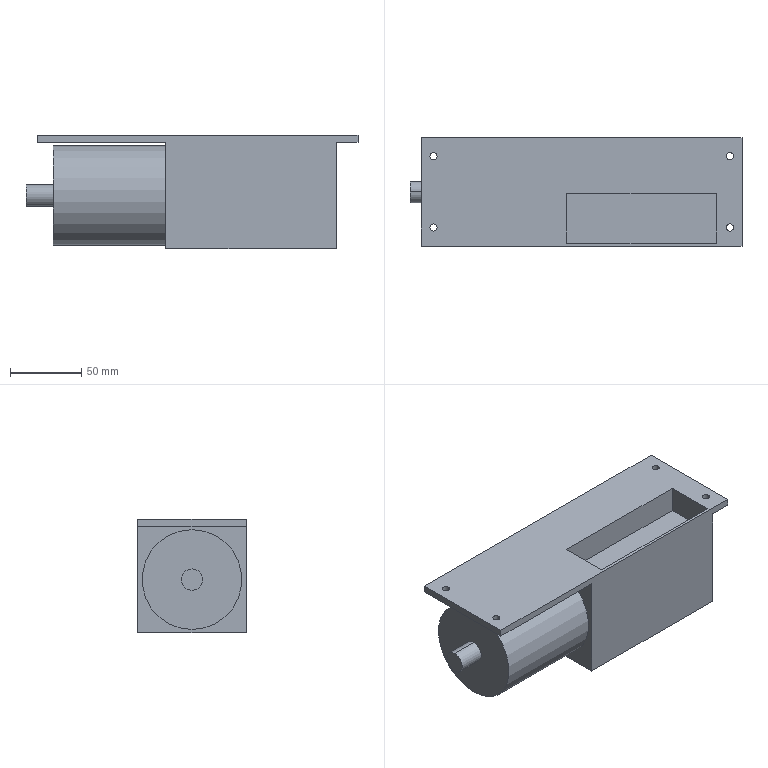Part | 1 solid | 29 faces | box 233 x 76 x 80 mm | volume 1006668 mm3 | plane 17 | cylinder 12 | commonest cylinder face diameters 5 x8 15 x2 70 x2
STEP:
#1=CARTESIAN_POINT('',(-120.5,0.,45.));
#2=VERTEX_POINT('',#1);
#3=CARTESIAN_POINT('',(-120.5,0.,30.));
#4=VERTEX_POINT('',#3);
#5=CARTESIAN_POINT('',(-120.5,0.,37.5));
#6=DIRECTION('',(-1.,0.,0.));
#7=DIRECTION('',(0.,0.,1.));
#8=AXIS2_PLACEMENT_3D('',#5,#6,#7);
#9=CIRCLE('',#8,7.5);
#10=EDGE_CURVE('',#2,#4,#9,.T.);
#11=ORIENTED_EDGE('',*,*,#10,.F.);
#12=CARTESIAN_POINT('',(-101.5,0.,45.));
#13=VERTEX_POINT('',#12);
#14=CARTESIAN_POINT('',(-120.5,0.,45.));
#15=DIRECTION('',(1.,0.,0.));
#16=VECTOR('',#15,1000.);
#17=LINE('',#14,#16);
#18=EDGE_CURVE('',#2,#13,#17,.T.);
#19=ORIENTED_EDGE('',*,*,#18,.T.);
#20=CARTESIAN_POINT('',(-101.5,0.,30.));
#21=VERTEX_POINT('',#20);
#22=CARTESIAN_POINT('',(-101.5,0.,37.5));
#23=DIRECTION('',(-1.,0.,0.));
#24=DIRECTION('',(0.,0.,1.));
#25=AXIS2_PLACEMENT_3D('',#22,#23,#24);
#26=CIRCLE('',#25,7.5);
#27=EDGE_CURVE('',#13,#21,#26,.T.);
#28=ORIENTED_EDGE('',*,*,#27,.T.);
#29=CARTESIAN_POINT('',(-120.5,0.,30.));
#30=DIRECTION('',(1.,0.,0.));
#31=VECTOR('',#30,1000.);
#32=LINE('',#29,#31);
#33=EDGE_CURVE('',#4,#21,#32,.T.);
#34=ORIENTED_EDGE('',*,*,#33,.F.);
#35=EDGE_LOOP('',(#11,#19,#28,#34));
#36=FACE_OUTER_BOUND('',#35,.T.);
#37=CARTESIAN_POINT('',(-120.5,0.,37.5));
#38=DIRECTION('',(1.,0.,0.));
#39=DIRECTION('',(0.,0.,-1.));
#40=AXIS2_PLACEMENT_3D('',#37,#38,#39);
#41=CYLINDRICAL_SURFACE('',#40,7.5);
#42=ADVANCED_FACE('',(#36),#41,.T.);
#43=CARTESIAN_POINT('',(-101.5,0.,72.5));
#44=VERTEX_POINT('',#43);
#45=CARTESIAN_POINT('',(-101.5,0.,2.5));
#46=VERTEX_POINT('',#45);
#47=CARTESIAN_POINT('',(-101.5,0.,37.5));
#48=DIRECTION('',(-1.,0.,0.));
#49=DIRECTION('',(0.,0.,1.));
#50=AXIS2_PLACEMENT_3D('',#47,#48,#49);
#51=CIRCLE('',#50,35.);
#52=EDGE_CURVE('',#44,#46,#51,.T.);
#53=ORIENTED_EDGE('',*,*,#52,.F.);
#54=CARTESIAN_POINT('',(-22.5,0.,72.5));
#55=VERTEX_POINT('',#54);
#56=CARTESIAN_POINT('',(-101.5,0.,72.5));
#57=DIRECTION('',(1.,0.,0.));
#58=VECTOR('',#57,1000.);
#59=LINE('',#56,#58);
#60=EDGE_CURVE('',#44,#55,#59,.T.);
#61=ORIENTED_EDGE('',*,*,#60,.T.);
#62=CARTESIAN_POINT('',(-22.5,0.,2.5));
#63=VERTEX_POINT('',#62);
#64=CARTESIAN_POINT('',(-22.5,0.,37.5));
#65=DIRECTION('',(-1.,0.,0.));
#66=DIRECTION('',(0.,0.,-1.));
#67=AXIS2_PLACEMENT_3D('',#64,#65,#66);
#68=CIRCLE('',#67,35.);
#69=EDGE_CURVE('',#55,#63,#68,.T.);
#70=ORIENTED_EDGE('',*,*,#69,.T.);
#71=CARTESIAN_POINT('',(-101.5,0.,2.5));
#72=DIRECTION('',(1.,0.,0.));
#73=VECTOR('',#72,1000.);
#74=LINE('',#71,#73);
#75=EDGE_CURVE('',#46,#63,#74,.T.);
#76=ORIENTED_EDGE('',*,*,#75,.F.);
#77=EDGE_LOOP('',(#53,#61,#70,#76));
#78=FACE_OUTER_BOUND('',#77,.T.);
#79=CARTESIAN_POINT('',(-101.5,0.,37.5));
#80=DIRECTION('',(1.,0.,0.));
#81=DIRECTION('',(0.,0.,-1.));
#82=AXIS2_PLACEMENT_3D('',#79,#80,#81);
#83=CYLINDRICAL_SURFACE('',#82,35.);
#84=ADVANCED_FACE('',(#78),#83,.T.);
#85=CARTESIAN_POINT('',(-106.5,25.,80.));
#86=VERTEX_POINT('',#85);
#87=CARTESIAN_POINT('',(-101.5,25.,80.));
#88=VERTEX_POINT('',#87);
#89=CARTESIAN_POINT('',(-104.,25.,80.));
#90=DIRECTION('',(0.,0.,1.));
#91=DIRECTION('',(1.,0.,0.));
#92=AXIS2_PLACEMENT_3D('',#89,#90,#91);
#93=CIRCLE('',#92,2.5);
#94=EDGE_CURVE('',#86,#88,#93,.T.);
#95=ORIENTED_EDGE('',*,*,#94,.T.);
#96=CARTESIAN_POINT('',(-101.5,25.,75.));
#97=VERTEX_POINT('',#96);
#98=CARTESIAN_POINT('',(-101.5,25.,90.));
#99=DIRECTION('',(0.,0.,-1.));
#100=VECTOR('',#99,1000.);
#101=LINE('',#98,#100);
#102=EDGE_CURVE('',#88,#97,#101,.T.);
#103=ORIENTED_EDGE('',*,*,#102,.T.);
#104=CARTESIAN_POINT('',(-106.5,25.,75.));
#105=VERTEX_POINT('',#104);
#106=CARTESIAN_POINT('',(-104.,25.,75.));
#107=DIRECTION('',(0.,0.,-1.));
#108=DIRECTION('',(-1.,0.,0.));
#109=AXIS2_PLACEMENT_3D('',#106,#107,#108);
#110=CIRCLE('',#109,2.5);
#111=EDGE_CURVE('',#97,#105,#110,.T.);
#112=ORIENTED_EDGE('',*,*,#111,.T.);
#113=CARTESIAN_POINT('',(-106.5,25.,90.));
#114=DIRECTION('',(0.,0.,-1.));
#115=VECTOR('',#114,1000.);
#116=LINE('',#113,#115);
#117=EDGE_CURVE('',#86,#105,#116,.T.);
#118=ORIENTED_EDGE('',*,*,#117,.F.);
#119=EDGE_LOOP('',(#95,#103,#112,#118));
#120=FACE_OUTER_BOUND('',#119,.T.);
#121=CARTESIAN_POINT('',(-104.,25.,90.));
#122=DIRECTION('',(0.,0.,-1.));
#123=DIRECTION('',(-1.,0.,0.));
#124=AXIS2_PLACEMENT_3D('',#121,#122,#123);
#125=CYLINDRICAL_SURFACE('',#124,2.5);
#126=ADVANCED_FACE('',(#120),#125,.F.);
#127=CARTESIAN_POINT('',(-106.5,-25.,80.));
#128=VERTEX_POINT('',#127);
#129=CARTESIAN_POINT('',(-101.5,-25.,80.));
#130=VERTEX_POINT('',#129);
#131=CARTESIAN_POINT('',(-104.,-25.,80.));
#132=DIRECTION('',(0.,0.,1.));
#133=DIRECTION('',(1.,0.,0.));
#134=AXIS2_PLACEMENT_3D('',#131,#132,#133);
#135=CIRCLE('',#134,2.5);
#136=EDGE_CURVE('',#128,#130,#135,.T.);
#137=ORIENTED_EDGE('',*,*,#136,.T.);
#138=CARTESIAN_POINT('',(-101.5,-25.,75.));
#139=VERTEX_POINT('',#138);
#140=CARTESIAN_POINT('',(-101.5,-25.,90.));
#141=DIRECTION('',(0.,0.,-1.));
#142=VECTOR('',#141,1000.);
#143=LINE('',#140,#142);
#144=EDGE_CURVE('',#130,#139,#143,.T.);
#145=ORIENTED_EDGE('',*,*,#144,.T.);
#146=CARTESIAN_POINT('',(-106.5,-25.,75.));
#147=VERTEX_POINT('',#146);
#148=CARTESIAN_POINT('',(-104.,-25.,75.));
#149=DIRECTION('',(0.,0.,-1.));
#150=DIRECTION('',(-1.,0.,0.));
#151=AXIS2_PLACEMENT_3D('',#148,#149,#150);
#152=CIRCLE('',#151,2.5);
#153=EDGE_CURVE('',#139,#147,#152,.T.);
#154=ORIENTED_EDGE('',*,*,#153,.T.);
#155=CARTESIAN_POINT('',(-106.5,-25.,90.));
#156=DIRECTION('',(0.,0.,-1.));
#157=VECTOR('',#156,1000.);
#158=LINE('',#155,#157);
#159=EDGE_CURVE('',#128,#147,#158,.T.);
#160=ORIENTED_EDGE('',*,*,#159,.F.);
#161=EDGE_LOOP('',(#137,#145,#154,#160));
#162=FACE_OUTER_BOUND('',#161,.T.);
#163=CARTESIAN_POINT('',(-104.,-25.,90.));
#164=DIRECTION('',(0.,0.,-1.));
#165=DIRECTION('',(-1.,0.,0.));
#166=AXIS2_PLACEMENT_3D('',#163,#164,#165);
#167=CYLINDRICAL_SURFACE('',#166,2.5);
#168=ADVANCED_FACE('',(#162),#167,.F.);
#169=CARTESIAN_POINT('',(101.5,-25.,80.));
#170=VERTEX_POINT('',#169);
#171=CARTESIAN_POINT('',(106.5,-25.,80.));
#172=VERTEX_POINT('',#171);
#173=CARTESIAN_POINT('',(104.,-25.,80.));
#174=DIRECTION('',(0.,0.,1.));
#175=DIRECTION('',(1.,0.,0.));
#176=AXIS2_PLACEMENT_3D('',#173,#174,#175);
#177=CIRCLE('',#176,2.5);
#178=EDGE_CURVE('',#170,#172,#177,.T.);
#179=ORIENTED_EDGE('',*,*,#178,.T.);
#180=CARTESIAN_POINT('',(106.5,-25.,75.));
#181=VERTEX_POINT('',#180);
#182=CARTESIAN_POINT('',(106.5,-25.,90.));
#183=DIRECTION('',(0.,0.,-1.));
#184=VECTOR('',#183,1000.);
#185=LINE('',#182,#184);
#186=EDGE_CURVE('',#172,#181,#185,.T.);
#187=ORIENTED_EDGE('',*,*,#186,.T.);
#188=CARTESIAN_POINT('',(101.5,-25.,75.));
#189=VERTEX_POINT('',#188);
#190=CARTESIAN_POINT('',(104.,-25.,75.));
#191=DIRECTION('',(0.,0.,-1.));
#192=DIRECTION('',(-1.,0.,0.));
#193=AXIS2_PLACEMENT_3D('',#190,#191,#192);
#194=CIRCLE('',#193,2.5);
#195=EDGE_CURVE('',#181,#189,#194,.T.);
#196=ORIENTED_EDGE('',*,*,#195,.T.);
#197=CARTESIAN_POINT('',(101.5,-25.,90.));
#198=DIRECTION('',(0.,0.,-1.));
#199=VECTOR('',#198,1000.);
#200=LINE('',#197,#199);
#201=EDGE_CURVE('',#170,#189,#200,.T.);
#202=ORIENTED_EDGE('',*,*,#201,.F.);
#203=EDGE_LOOP('',(#179,#187,#196,#202));
#204=FACE_OUTER_BOUND('',#203,.T.);
#205=CARTESIAN_POINT('',(104.,-25.,90.));
#206=DIRECTION('',(0.,0.,-1.));
#207=DIRECTION('',(-1.,0.,0.));
#208=AXIS2_PLACEMENT_3D('',#205,#206,#207);
#209=CYLINDRICAL_SURFACE('',#208,2.5);
#210=ADVANCED_FACE('',(#204),#209,.F.);
#211=CARTESIAN_POINT('',(101.5,25.,80.));
#212=VERTEX_POINT('',#211);
#213=CARTESIAN_POINT('',(106.5,25.,80.));
#214=VERTEX_POINT('',#213);
#215=CARTESIAN_POINT('',(104.,25.,80.));
#216=DIRECTION('',(0.,0.,1.));
#217=DIRECTION('',(1.,0.,0.));
#218=AXIS2_PLACEMENT_3D('',#215,#216,#217);
#219=CIRCLE('',#218,2.5);
#220=EDGE_CURVE('',#212,#214,#219,.T.);
#221=ORIENTED_EDGE('',*,*,#220,.T.);
#222=CARTESIAN_POINT('',(106.5,25.,75.));
#223=VERTEX_POINT('',#222);
#224=CARTESIAN_POINT('',(106.5,25.,90.));
#225=DIRECTION('',(0.,0.,-1.));
#226=VECTOR('',#225,1000.);
#227=LINE('',#224,#226);
#228=EDGE_CURVE('',#214,#223,#227,.T.);
#229=ORIENTED_EDGE('',*,*,#228,.T.);
#230=CARTESIAN_POINT('',(101.5,25.,75.));
#231=VERTEX_POINT('',#230);
#232=CARTESIAN_POINT('',(104.,25.,75.));
#233=DIRECTION('',(0.,0.,-1.));
#234=DIRECTION('',(-1.,0.,0.));
#235=AXIS2_PLACEMENT_3D('',#232,#233,#234);
#236=CIRCLE('',#235,2.5);
#237=EDGE_CURVE('',#223,#231,#236,.T.);
#238=ORIENTED_EDGE('',*,*,#237,.T.);
#239=CARTESIAN_POINT('',(101.5,25.,90.));
#240=DIRECTION('',(0.,0.,-1.));
#241=VECTOR('',#240,1000.);
#242=LINE('',#239,#241);
#243=EDGE_CURVE('',#212,#231,#242,.T.);
#244=ORIENTED_EDGE('',*,*,#243,.F.);
#245=EDGE_LOOP('',(#221,#229,#238,#244));
#246=FACE_OUTER_BOUND('',#245,.T.);
#247=CARTESIAN_POINT('',(104.,25.,90.));
#248=DIRECTION('',(0.,0.,-1.));
#249=DIRECTION('',(-1.,0.,0.));
#250=AXIS2_PLACEMENT_3D('',#247,#248,#249);
#251=CYLINDRICAL_SURFACE('',#250,2.5);
#252=ADVANCED_FACE('',(#246),#251,.F.);
#253=CARTESIAN_POINT('',(112.5,-38.,80.));
#254=VERTEX_POINT('',#253);
#255=CARTESIAN_POINT('',(112.5,-38.,75.));
#256=VERTEX_POINT('',#255);
#257=CARTESIAN_POINT('',(112.5,-38.,80.));
#258=DIRECTION('',(0.,0.,-1.));
#259=VECTOR('',#258,1000.);
#260=LINE('',#257,#259);
#261=EDGE_CURVE('',#254,#256,#260,.T.);
#262=ORIENTED_EDGE('',*,*,#261,.T.);
#263=CARTESIAN_POINT('',(112.5,38.,75.));
#264=VERTEX_POINT('',#263);
#265=CARTESIAN_POINT('',(112.5,38.,75.));
#266=DIRECTION('',(0.,-1.,0.));
#267=VECTOR('',#266,1000.);
#268=LINE('',#265,#267);
#269=EDGE_CURVE('',#264,#256,#268,.T.);
#270=ORIENTED_EDGE('',*,*,#269,.F.);
#271=CARTESIAN_POINT('',(112.5,38.,80.));
#272=VERTEX_POINT('',#271);
#273=CARTESIAN_POINT('',(112.5,38.,80.));
#274=DIRECTION('',(0.,0.,-1.));
#275=VECTOR('',#274,1000.);
#276=LINE('',#273,#275);
#277=EDGE_CURVE('',#272,#264,#276,.T.);
#278=ORIENTED_EDGE('',*,*,#277,.F.);
#279=CARTESIAN_POINT('',(112.5,38.,80.));
#280=DIRECTION('',(0.,1.,0.));
#281=VECTOR('',#280,1000.);
#282=LINE('',#279,#281);
#283=EDGE_CURVE('',#254,#272,#282,.T.);
#284=ORIENTED_EDGE('',*,*,#283,.F.);
#285=EDGE_LOOP('',(#262,#270,#278,#284));
#286=FACE_OUTER_BOUND('',#285,.T.);
#287=CARTESIAN_POINT('',(112.5,38.,80.));
#288=DIRECTION('',(-1.,0.,0.));
#289=DIRECTION('',(0.,-1.,0.));
#290=AXIS2_PLACEMENT_3D('',#287,#288,#289);
#291=PLANE('',#290);
#292=ADVANCED_FACE('',(#286),#291,.F.);
#293=ORIENTED_EDGE('',*,*,#277,.T.);
#294=CARTESIAN_POINT('',(97.5,38.,75.));
#295=VERTEX_POINT('',#294);
#296=CARTESIAN_POINT('',(97.5,38.,75.));
#297=DIRECTION('',(1.,0.,0.));
#298=VECTOR('',#297,1000.);
#299=LINE('',#296,#298);
#300=EDGE_CURVE('',#295,#264,#299,.T.);
#301=ORIENTED_EDGE('',*,*,#300,.F.);
#302=CARTESIAN_POINT('',(97.5,38.,0.));
#303=VERTEX_POINT('',#302);
#304=CARTESIAN_POINT('',(97.5,38.,0.));
#305=DIRECTION('',(0.,0.,1.));
#306=VECTOR('',#305,1000.);
#307=LINE('',#304,#306);
#308=EDGE_CURVE('',#303,#295,#307,.T.);
#309=ORIENTED_EDGE('',*,*,#308,.F.);
#310=CARTESIAN_POINT('',(-22.5,38.,0.));
#311=VERTEX_POINT('',#310);
#312=CARTESIAN_POINT('',(-112.5,38.,0.));
#313=DIRECTION('',(-1.,0.,0.));
#314=VECTOR('',#313,1000.);
#315=LINE('',#312,#314);
#316=EDGE_CURVE('',#303,#311,#315,.T.);
#317=ORIENTED_EDGE('',*,*,#316,.T.);
#318=CARTESIAN_POINT('',(-22.5,38.,75.));
#319=VERTEX_POINT('',#318);
#320=CARTESIAN_POINT('',(-22.5,38.,0.));
#321=DIRECTION('',(0.,0.,-1.));
#322=VECTOR('',#321,1000.);
#323=LINE('',#320,#322);
#324=EDGE_CURVE('',#319,#311,#323,.T.);
#325=ORIENTED_EDGE('',*,*,#324,.F.);
#326=CARTESIAN_POINT('',(-112.5,38.,75.));
#327=VERTEX_POINT('',#326);
#328=CARTESIAN_POINT('',(-22.5,38.,75.));
#329=DIRECTION('',(-1.,0.,0.));
#330=VECTOR('',#329,1000.);
#331=LINE('',#328,#330);
#332=EDGE_CURVE('',#319,#327,#331,.T.);
#333=ORIENTED_EDGE('',*,*,#332,.T.);
#334=CARTESIAN_POINT('',(-112.5,38.,80.));
#335=VERTEX_POINT('',#334);
#336=CARTESIAN_POINT('',(-112.5,38.,80.));
#337=DIRECTION('',(0.,0.,-1.));
#338=VECTOR('',#337,1000.);
#339=LINE('',#336,#338);
#340=EDGE_CURVE('',#335,#327,#339,.T.);
#341=ORIENTED_EDGE('',*,*,#340,.F.);
#342=CARTESIAN_POINT('',(-112.5,38.,80.));
#343=DIRECTION('',(-1.,0.,0.));
#344=VECTOR('',#343,1000.);
#345=LINE('',#342,#344);
#346=EDGE_CURVE('',#272,#335,#345,.T.);
#347=ORIENTED_EDGE('',*,*,#346,.F.);
#348=EDGE_LOOP('',(#293,#301,#309,#317,#325,#333,#341,#347));
#349=FACE_OUTER_BOUND('',#348,.T.);
#350=CARTESIAN_POINT('',(-112.5,38.,80.));
#351=DIRECTION('',(0.,-1.,0.));
#352=DIRECTION('',(0.,0.,-1.));
#353=AXIS2_PLACEMENT_3D('',#350,#351,#352);
#354=PLANE('',#353);
#355=ADVANCED_FACE('',(#349),#354,.F.);
#356=ORIENTED_EDGE('',*,*,#340,.T.);
#357=CARTESIAN_POINT('',(-112.5,-38.,75.));
#358=VERTEX_POINT('',#357);
#359=CARTESIAN_POINT('',(-112.5,-38.,75.));
#360=DIRECTION('',(0.,1.,0.));
#361=VECTOR('',#360,1000.);
#362=LINE('',#359,#361);
#363=EDGE_CURVE('',#358,#327,#362,.T.);
#364=ORIENTED_EDGE('',*,*,#363,.F.);
#365=CARTESIAN_POINT('',(-112.5,-38.,80.));
#366=VERTEX_POINT('',#365);
#367=CARTESIAN_POINT('',(-112.5,-38.,80.));
#368=DIRECTION('',(0.,0.,-1.));
#369=VECTOR('',#368,1000.);
#370=LINE('',#367,#369);
#371=EDGE_CURVE('',#366,#358,#370,.T.);
#372=ORIENTED_EDGE('',*,*,#371,.F.);
#373=CARTESIAN_POINT('',(-112.5,38.,80.));
#374=DIRECTION('',(0.,-1.,0.));
#375=VECTOR('',#374,1000.);
#376=LINE('',#373,#375);
#377=EDGE_CURVE('',#335,#366,#376,.T.);
#378=ORIENTED_EDGE('',*,*,#377,.F.);
#379=EDGE_LOOP('',(#356,#364,#372,#378));
#380=FACE_OUTER_BOUND('',#379,.T.);
#381=CARTESIAN_POINT('',(-112.5,38.,80.));
#382=DIRECTION('',(1.,0.,0.));
#383=DIRECTION('',(0.,0.,-1.));
#384=AXIS2_PLACEMENT_3D('',#381,#382,#383);
#385=PLANE('',#384);
#386=ADVANCED_FACE('',(#380),#385,.F.);
#387=CARTESIAN_POINT('',(97.5,-38.,75.));
#388=VERTEX_POINT('',#387);
#389=CARTESIAN_POINT('',(97.5,-38.,0.));
#390=VERTEX_POINT('',#389);
#391=CARTESIAN_POINT('',(97.5,-38.,0.));
#392=DIRECTION('',(0.,0.,-1.));
#393=VECTOR('',#392,1000.);
#394=LINE('',#391,#393);
#395=EDGE_CURVE('',#388,#390,#394,.T.);
#396=ORIENTED_EDGE('',*,*,#395,.F.);
#397=CARTESIAN_POINT('',(97.5,-38.,75.));
#398=DIRECTION('',(1.,0.,0.));
#399=VECTOR('',#398,1000.);
#400=LINE('',#397,#399);
#401=EDGE_CURVE('',#388,#256,#400,.T.);
#402=ORIENTED_EDGE('',*,*,#401,.T.);
#403=ORIENTED_EDGE('',*,*,#261,.F.);
#404=CARTESIAN_POINT('',(-112.5,-38.,80.));
#405=DIRECTION('',(1.,0.,0.));
#406=VECTOR('',#405,1000.);
#407=LINE('',#404,#406);
#408=EDGE_CURVE('',#366,#254,#407,.T.);
#409=ORIENTED_EDGE('',*,*,#408,.F.);
#410=ORIENTED_EDGE('',*,*,#371,.T.);
#411=CARTESIAN_POINT('',(-22.5,-38.,75.));
#412=VERTEX_POINT('',#411);
#413=CARTESIAN_POINT('',(-22.5,-38.,75.));
#414=DIRECTION('',(-1.,0.,0.));
#415=VECTOR('',#414,1000.);
#416=LINE('',#413,#415);
#417=EDGE_CURVE('',#412,#358,#416,.T.);
#418=ORIENTED_EDGE('',*,*,#417,.F.);
#419=CARTESIAN_POINT('',(-22.5,-38.,0.));
#420=VERTEX_POINT('',#419);
#421=CARTESIAN_POINT('',(-22.5,-38.,0.));
#422=DIRECTION('',(0.,0.,1.));
#423=VECTOR('',#422,1000.);
#424=LINE('',#421,#423);
#425=EDGE_CURVE('',#420,#412,#424,.T.);
#426=ORIENTED_EDGE('',*,*,#425,.F.);
#427=CARTESIAN_POINT('',(-112.5,-38.,0.));
#428=DIRECTION('',(1.,0.,0.));
#429=VECTOR('',#428,1000.);
#430=LINE('',#427,#429);
#431=EDGE_CURVE('',#420,#390,#430,.T.);
#432=ORIENTED_EDGE('',*,*,#431,.T.);
#433=EDGE_LOOP('',(#396,#402,#403,#409,#410,#418,#426,#432));
#434=FACE_OUTER_BOUND('',#433,.T.);
#435=CARTESIAN_POINT('',(-112.5,-38.,80.));
#436=DIRECTION('',(0.,1.,0.));
#437=DIRECTION('',(0.,0.,1.));
#438=AXIS2_PLACEMENT_3D('',#435,#436,#437);
#439=PLANE('',#438);
#440=ADVANCED_FACE('',(#434),#439,.F.);
#441=CARTESIAN_POINT('',(-10.5,-1.,80.));
#442=VERTEX_POINT('',#441);
#443=CARTESIAN_POINT('',(-10.5,-36.,80.));
#444=VERTEX_POINT('',#443);
#445=CARTESIAN_POINT('',(-10.5,-1.,80.));
#446=DIRECTION('',(0.,-1.,0.));
#447=VECTOR('',#446,1000.);
#448=LINE('',#445,#447);
#449=EDGE_CURVE('',#442,#444,#448,.T.);
#450=ORIENTED_EDGE('',*,*,#449,.F.);
#451=CARTESIAN_POINT('',(94.5,-1.,80.));
#452=VERTEX_POINT('',#451);
#453=CARTESIAN_POINT('',(-10.5,-1.,80.));
#454=DIRECTION('',(-1.,0.,0.));
#455=VECTOR('',#454,1000.);
#456=LINE('',#453,#455);
#457=EDGE_CURVE('',#452,#442,#456,.T.);
#458=ORIENTED_EDGE('',*,*,#457,.F.);
#459=CARTESIAN_POINT('',(94.5,-36.,80.));
#460=VERTEX_POINT('',#459);
#461=CARTESIAN_POINT('',(94.5,-1.,80.));
#462=DIRECTION('',(0.,1.,0.));
#463=VECTOR('',#462,1000.);
#464=LINE('',#461,#463);
#465=EDGE_CURVE('',#460,#452,#464,.T.);
#466=ORIENTED_EDGE('',*,*,#465,.F.);
#467=CARTESIAN_POINT('',(-10.5,-36.,80.));
#468=DIRECTION('',(1.,0.,0.));
#469=VECTOR('',#468,1000.);
#470=LINE('',#467,#469);
#471=EDGE_CURVE('',#444,#460,#470,.T.);
#472=ORIENTED_EDGE('',*,*,#471,.F.);
#473=EDGE_LOOP('',(#450,#458,#466,#472));
#474=FACE_BOUND('',#473,.T.);
#475=ORIENTED_EDGE('',*,*,#94,.F.);
#476=CARTESIAN_POINT('',(-104.,25.,80.));
#477=DIRECTION('',(0.,0.,1.));
#478=DIRECTION('',(1.,0.,0.));
#479=AXIS2_PLACEMENT_3D('',#476,#477,#478);
#480=CIRCLE('',#479,2.5);
#481=EDGE_CURVE('',#88,#86,#480,.T.);
#482=ORIENTED_EDGE('',*,*,#481,.F.);
#483=EDGE_LOOP('',(#475,#482));
#484=FACE_BOUND('',#483,.T.);
#485=ORIENTED_EDGE('',*,*,#178,.F.);
#486=CARTESIAN_POINT('',(104.,-25.,80.));
#487=DIRECTION('',(0.,0.,1.));
#488=DIRECTION('',(1.,0.,0.));
#489=AXIS2_PLACEMENT_3D('',#486,#487,#488);
#490=CIRCLE('',#489,2.5);
#491=EDGE_CURVE('',#172,#170,#490,.T.);
#492=ORIENTED_EDGE('',*,*,#491,.F.);
#493=EDGE_LOOP('',(#485,#492));
#494=FACE_BOUND('',#493,.T.);
#495=ORIENTED_EDGE('',*,*,#220,.F.);
#496=CARTESIAN_POINT('',(104.,25.,80.));
#497=DIRECTION('',(0.,0.,1.));
#498=DIRECTION('',(1.,0.,0.));
#499=AXIS2_PLACEMENT_3D('',#496,#497,#498);
#500=CIRCLE('',#499,2.5);
#501=EDGE_CURVE('',#214,#212,#500,.T.);
#502=ORIENTED_EDGE('',*,*,#501,.F.);
#503=EDGE_LOOP('',(#495,#502));
#504=FACE_BOUND('',#503,.T.);
#505=ORIENTED_EDGE('',*,*,#136,.F.);
#506=CARTESIAN_POINT('',(-104.,-25.,80.));
#507=DIRECTION('',(0.,0.,1.));
#508=DIRECTION('',(1.,0.,0.));
#509=AXIS2_PLACEMENT_3D('',#506,#507,#508);
#510=CIRCLE('',#509,2.5);
#511=EDGE_CURVE('',#130,#128,#510,.T.);
#512=ORIENTED_EDGE('',*,*,#511,.F.);
#513=EDGE_LOOP('',(#505,#512));
#514=FACE_BOUND('',#513,.T.);
#515=ORIENTED_EDGE('',*,*,#283,.T.);
#516=ORIENTED_EDGE('',*,*,#346,.T.);
#517=ORIENTED_EDGE('',*,*,#377,.T.);
#518=ORIENTED_EDGE('',*,*,#408,.T.);
#519=EDGE_LOOP('',(#515,#516,#517,#518));
#520=FACE_OUTER_BOUND('',#519,.T.);
#521=CARTESIAN_POINT('',(0.,0.,80.));
#522=DIRECTION('',(0.,0.,1.));
#523=DIRECTION('',(1.,0.,0.));
#524=AXIS2_PLACEMENT_3D('',#521,#522,#523);
#525=PLANE('',#524);
#526=ADVANCED_FACE('',(#474,#484,#494,#504,#514,#520),#525,.T.);
#527=ORIENTED_EDGE('',*,*,#316,.F.);
#528=CARTESIAN_POINT('',(97.5,38.,0.));
#529=DIRECTION('',(0.,1.,0.));
#530=VECTOR('',#529,1000.);
#531=LINE('',#528,#530);
#532=EDGE_CURVE('',#390,#303,#531,.T.);
#533=ORIENTED_EDGE('',*,*,#532,.F.);
#534=ORIENTED_EDGE('',*,*,#431,.F.);
#535=CARTESIAN_POINT('',(-22.5,-38.,0.));
#536=DIRECTION('',(0.,-1.,0.));
#537=VECTOR('',#536,1000.);
#538=LINE('',#535,#537);
#539=EDGE_CURVE('',#311,#420,#538,.T.);
#540=ORIENTED_EDGE('',*,*,#539,.F.);
#541=EDGE_LOOP('',(#527,#533,#534,#540));
#542=FACE_OUTER_BOUND('',#541,.T.);
#543=CARTESIAN_POINT('',(0.,0.,0.));
#544=DIRECTION('',(0.,0.,1.));
#545=DIRECTION('',(1.,0.,0.));
#546=AXIS2_PLACEMENT_3D('',#543,#544,#545);
#547=PLANE('',#546);
#548=ADVANCED_FACE('',(#542),#547,.F.);
#549=CARTESIAN_POINT('',(-104.,25.,75.));
#550=DIRECTION('',(0.,0.,-1.));
#551=DIRECTION('',(-1.,0.,0.));
#552=AXIS2_PLACEMENT_3D('',#549,#550,#551);
#553=CIRCLE('',#552,2.5);
#554=EDGE_CURVE('',#105,#97,#553,.T.);
#555=ORIENTED_EDGE('',*,*,#554,.F.);
#556=ORIENTED_EDGE('',*,*,#111,.F.);
#557=EDGE_LOOP('',(#555,#556));
#558=FACE_BOUND('',#557,.T.);
#559=CARTESIAN_POINT('',(-104.,-25.,75.));
#560=DIRECTION('',(0.,0.,-1.));
#561=DIRECTION('',(-1.,0.,0.));
#562=AXIS2_PLACEMENT_3D('',#559,#560,#561);
#563=CIRCLE('',#562,2.5);
#564=EDGE_CURVE('',#147,#139,#563,.T.);
#565=ORIENTED_EDGE('',*,*,#564,.F.);
#566=ORIENTED_EDGE('',*,*,#153,.F.);
#567=EDGE_LOOP('',(#565,#566));
#568=FACE_BOUND('',#567,.T.);
#569=ORIENTED_EDGE('',*,*,#363,.T.);
#570=ORIENTED_EDGE('',*,*,#332,.F.);
#571=CARTESIAN_POINT('',(-22.5,-38.,75.));
#572=DIRECTION('',(0.,1.,0.));
#573=VECTOR('',#572,1000.);
#574=LINE('',#571,#573);
#575=EDGE_CURVE('',#412,#319,#574,.T.);
#576=ORIENTED_EDGE('',*,*,#575,.F.);
#577=ORIENTED_EDGE('',*,*,#417,.T.);
#578=EDGE_LOOP('',(#569,#570,#576,#577));
#579=FACE_OUTER_BOUND('',#578,.T.);
#580=CARTESIAN_POINT('',(-22.5,-38.,75.));
#581=DIRECTION('',(0.,0.,1.));
#582=DIRECTION('',(1.,0.,0.));
#583=AXIS2_PLACEMENT_3D('',#580,#581,#582);
#584=PLANE('',#583);
#585=ADVANCED_FACE('',(#558,#568,#579),#584,.F.);
#586=CARTESIAN_POINT('',(-22.5,0.,37.5));
#587=DIRECTION('',(-1.,0.,0.));
#588=DIRECTION('',(0.,0.,-1.));
#589=AXIS2_PLACEMENT_3D('',#586,#587,#588);
#590=CIRCLE('',#589,35.);
#591=EDGE_CURVE('',#63,#55,#590,.T.);
#592=ORIENTED_EDGE('',*,*,#591,.F.);
#593=ORIENTED_EDGE('',*,*,#69,.F.);
#594=EDGE_LOOP('',(#592,#593));
#595=FACE_BOUND('',#594,.T.);
#596=ORIENTED_EDGE('',*,*,#539,.T.);
#597=ORIENTED_EDGE('',*,*,#425,.T.);
#598=ORIENTED_EDGE('',*,*,#575,.T.);
#599=ORIENTED_EDGE('',*,*,#324,.T.);
#600=EDGE_LOOP('',(#596,#597,#598,#599));
#601=FACE_OUTER_BOUND('',#600,.T.);
#602=CARTESIAN_POINT('',(-22.5,0.,0.));
#603=DIRECTION('',(1.,0.,0.));
#604=DIRECTION('',(0.,0.,-1.));
#605=AXIS2_PLACEMENT_3D('',#602,#603,#604);
#606=PLANE('',#605);
#607=ADVANCED_FACE('',(#595,#601),#606,.F.);
#608=CARTESIAN_POINT('',(104.,-25.,75.));
#609=DIRECTION('',(0.,0.,-1.));
#610=DIRECTION('',(-1.,0.,0.));
#611=AXIS2_PLACEMENT_3D('',#608,#609,#610);
#612=CIRCLE('',#611,2.5);
#613=EDGE_CURVE('',#189,#181,#612,.T.);
#614=ORIENTED_EDGE('',*,*,#613,.F.);
#615=ORIENTED_EDGE('',*,*,#195,.F.);
#616=EDGE_LOOP('',(#614,#615));
#617=FACE_BOUND('',#616,.T.);
#618=CARTESIAN_POINT('',(104.,25.,75.));
#619=DIRECTION('',(0.,0.,-1.));
#620=DIRECTION('',(-1.,0.,0.));
#621=AXIS2_PLACEMENT_3D('',#618,#619,#620);
#622=CIRCLE('',#621,2.5);
#623=EDGE_CURVE('',#231,#223,#622,.T.);
#624=ORIENTED_EDGE('',*,*,#623,.F.);
#625=ORIENTED_EDGE('',*,*,#237,.F.);
#626=EDGE_LOOP('',(#624,#625));
#627=FACE_BOUND('',#626,.T.);
#628=ORIENTED_EDGE('',*,*,#269,.T.);
#629=ORIENTED_EDGE('',*,*,#401,.F.);
#630=CARTESIAN_POINT('',(97.5,38.,75.));
#631=DIRECTION('',(0.,-1.,0.));
#632=VECTOR('',#631,1000.);
#633=LINE('',#630,#632);
#634=EDGE_CURVE('',#295,#388,#633,.T.);
#635=ORIENTED_EDGE('',*,*,#634,.F.);
#636=ORIENTED_EDGE('',*,*,#300,.T.);
#637=EDGE_LOOP('',(#628,#629,#635,#636));
#638=FACE_OUTER_BOUND('',#637,.T.);
#639=CARTESIAN_POINT('',(97.5,38.,75.));
#640=DIRECTION('',(0.,0.,1.));
#641=DIRECTION('',(0.,-1.,0.));
#642=AXIS2_PLACEMENT_3D('',#639,#640,#641);
#643=PLANE('',#642);
#644=ADVANCED_FACE('',(#617,#627,#638),#643,.F.);
#645=ORIENTED_EDGE('',*,*,#532,.T.);
#646=ORIENTED_EDGE('',*,*,#308,.T.);
#647=ORIENTED_EDGE('',*,*,#634,.T.);
#648=ORIENTED_EDGE('',*,*,#395,.T.);
#649=EDGE_LOOP('',(#645,#646,#647,#648));
#650=FACE_OUTER_BOUND('',#649,.T.);
#651=CARTESIAN_POINT('',(97.5,0.,0.));
#652=DIRECTION('',(-1.,0.,0.));
#653=DIRECTION('',(0.,-1.,0.));
#654=AXIS2_PLACEMENT_3D('',#651,#652,#653);
#655=PLANE('',#654);
#656=ADVANCED_FACE('',(#650),#655,.F.);
#657=ORIENTED_EDGE('',*,*,#228,.F.);
#658=ORIENTED_EDGE('',*,*,#501,.T.);
#659=ORIENTED_EDGE('',*,*,#243,.T.);
#660=ORIENTED_EDGE('',*,*,#623,.T.);
#661=EDGE_LOOP('',(#657,#658,#659,#660));
#662=FACE_OUTER_BOUND('',#661,.T.);
#663=CARTESIAN_POINT('',(104.,25.,90.));
#664=DIRECTION('',(0.,0.,-1.));
#665=DIRECTION('',(-1.,0.,0.));
#666=AXIS2_PLACEMENT_3D('',#663,#664,#665);
#667=CYLINDRICAL_SURFACE('',#666,2.5);
#668=ADVANCED_FACE('',(#662),#667,.F.);
#669=ORIENTED_EDGE('',*,*,#186,.F.);
#670=ORIENTED_EDGE('',*,*,#491,.T.);
#671=ORIENTED_EDGE('',*,*,#201,.T.);
#672=ORIENTED_EDGE('',*,*,#613,.T.);
#673=EDGE_LOOP('',(#669,#670,#671,#672));
#674=FACE_OUTER_BOUND('',#673,.T.);
#675=CARTESIAN_POINT('',(104.,-25.,90.));
#676=DIRECTION('',(0.,0.,-1.));
#677=DIRECTION('',(-1.,0.,0.));
#678=AXIS2_PLACEMENT_3D('',#675,#676,#677);
#679=CYLINDRICAL_SURFACE('',#678,2.5);
#680=ADVANCED_FACE('',(#674),#679,.F.);
#681=ORIENTED_EDGE('',*,*,#144,.F.);
#682=ORIENTED_EDGE('',*,*,#511,.T.);
#683=ORIENTED_EDGE('',*,*,#159,.T.);
#684=ORIENTED_EDGE('',*,*,#564,.T.);
#685=EDGE_LOOP('',(#681,#682,#683,#684));
#686=FACE_OUTER_BOUND('',#685,.T.);
#687=CARTESIAN_POINT('',(-104.,-25.,90.));
#688=DIRECTION('',(0.,0.,-1.));
#689=DIRECTION('',(-1.,0.,0.));
#690=AXIS2_PLACEMENT_3D('',#687,#688,#689);
#691=CYLINDRICAL_SURFACE('',#690,2.5);
#692=ADVANCED_FACE('',(#686),#691,.F.);
#693=ORIENTED_EDGE('',*,*,#102,.F.);
#694=ORIENTED_EDGE('',*,*,#481,.T.);
#695=ORIENTED_EDGE('',*,*,#117,.T.);
#696=ORIENTED_EDGE('',*,*,#554,.T.);
#697=EDGE_LOOP('',(#693,#694,#695,#696));
#698=FACE_OUTER_BOUND('',#697,.T.);
#699=CARTESIAN_POINT('',(-104.,25.,90.));
#700=DIRECTION('',(0.,0.,-1.));
#701=DIRECTION('',(-1.,0.,0.));
#702=AXIS2_PLACEMENT_3D('',#699,#700,#701);
#703=CYLINDRICAL_SURFACE('',#702,2.5);
#704=ADVANCED_FACE('',(#698),#703,.F.);
#705=ORIENTED_EDGE('',*,*,#60,.F.);
#706=CARTESIAN_POINT('',(-101.5,0.,37.5));
#707=DIRECTION('',(-1.,0.,0.));
#708=DIRECTION('',(0.,0.,1.));
#709=AXIS2_PLACEMENT_3D('',#706,#707,#708);
#710=CIRCLE('',#709,35.);
#711=EDGE_CURVE('',#46,#44,#710,.T.);
#712=ORIENTED_EDGE('',*,*,#711,.F.);
#713=ORIENTED_EDGE('',*,*,#75,.T.);
#714=ORIENTED_EDGE('',*,*,#591,.T.);
#715=EDGE_LOOP('',(#705,#712,#713,#714));
#716=FACE_OUTER_BOUND('',#715,.T.);
#717=CARTESIAN_POINT('',(-101.5,0.,37.5));
#718=DIRECTION('',(1.,0.,0.));
#719=DIRECTION('',(0.,0.,-1.));
#720=AXIS2_PLACEMENT_3D('',#717,#718,#719);
#721=CYLINDRICAL_SURFACE('',#720,35.);
#722=ADVANCED_FACE('',(#716),#721,.T.);
#723=CARTESIAN_POINT('',(-101.5,0.,37.5));
#724=DIRECTION('',(-1.,0.,0.));
#725=DIRECTION('',(0.,0.,1.));
#726=AXIS2_PLACEMENT_3D('',#723,#724,#725);
#727=CIRCLE('',#726,7.5);
#728=EDGE_CURVE('',#21,#13,#727,.T.);
#729=ORIENTED_EDGE('',*,*,#728,.F.);
#730=ORIENTED_EDGE('',*,*,#27,.F.);
#731=EDGE_LOOP('',(#729,#730));
#732=FACE_BOUND('',#731,.T.);
#733=ORIENTED_EDGE('',*,*,#711,.T.);
#734=ORIENTED_EDGE('',*,*,#52,.T.);
#735=EDGE_LOOP('',(#733,#734));
#736=FACE_OUTER_BOUND('',#735,.T.);
#737=CARTESIAN_POINT('',(-101.5,0.,37.5));
#738=DIRECTION('',(-1.,0.,0.));
#739=DIRECTION('',(0.,0.,1.));
#740=AXIS2_PLACEMENT_3D('',#737,#738,#739);
#741=PLANE('',#740);
#742=ADVANCED_FACE('',(#732,#736),#741,.T.);
#743=ORIENTED_EDGE('',*,*,#18,.F.);
#744=CARTESIAN_POINT('',(-120.5,0.,37.5));
#745=DIRECTION('',(-1.,0.,0.));
#746=DIRECTION('',(0.,0.,1.));
#747=AXIS2_PLACEMENT_3D('',#744,#745,#746);
#748=CIRCLE('',#747,7.5);
#749=EDGE_CURVE('',#4,#2,#748,.T.);
#750=ORIENTED_EDGE('',*,*,#749,.F.);
#751=ORIENTED_EDGE('',*,*,#33,.T.);
#752=ORIENTED_EDGE('',*,*,#728,.T.);
#753=EDGE_LOOP('',(#743,#750,#751,#752));
#754=FACE_OUTER_BOUND('',#753,.T.);
#755=CARTESIAN_POINT('',(-120.5,0.,37.5));
#756=DIRECTION('',(1.,0.,0.));
#757=DIRECTION('',(0.,0.,-1.));
#758=AXIS2_PLACEMENT_3D('',#755,#756,#757);
#759=CYLINDRICAL_SURFACE('',#758,7.5);
#760=ADVANCED_FACE('',(#754),#759,.T.);
#761=ORIENTED_EDGE('',*,*,#749,.T.);
#762=ORIENTED_EDGE('',*,*,#10,.T.);
#763=EDGE_LOOP('',(#761,#762));
#764=FACE_OUTER_BOUND('',#763,.T.);
#765=CARTESIAN_POINT('',(-120.5,0.,37.5));
#766=DIRECTION('',(-1.,0.,0.));
#767=DIRECTION('',(0.,0.,1.));
#768=AXIS2_PLACEMENT_3D('',#765,#766,#767);
#769=PLANE('',#768);
#770=ADVANCED_FACE('',(#764),#769,.T.);
#771=ORIENTED_EDGE('',*,*,#449,.T.);
#772=CARTESIAN_POINT('',(-10.5,-36.,61.));
#773=VERTEX_POINT('',#772);
#774=CARTESIAN_POINT('',(-10.5,-36.,61.));
#775=DIRECTION('',(0.,0.,1.));
#776=VECTOR('',#775,1000.);
#777=LINE('',#774,#776);
#778=EDGE_CURVE('',#773,#444,#777,.T.);
#779=ORIENTED_EDGE('',*,*,#778,.F.);
#780=CARTESIAN_POINT('',(-10.5,-1.,61.));
#781=VERTEX_POINT('',#780);
#782=CARTESIAN_POINT('',(-10.5,-1.,61.));
#783=DIRECTION('',(0.,-1.,0.));
#784=VECTOR('',#783,1000.);
#785=LINE('',#782,#784);
#786=EDGE_CURVE('',#781,#773,#785,.T.);
#787=ORIENTED_EDGE('',*,*,#786,.F.);
#788=CARTESIAN_POINT('',(-10.5,-1.,61.));
#789=DIRECTION('',(0.,0.,1.));
#790=VECTOR('',#789,1000.);
#791=LINE('',#788,#790);
#792=EDGE_CURVE('',#781,#442,#791,.T.);
#793=ORIENTED_EDGE('',*,*,#792,.T.);
#794=EDGE_LOOP('',(#771,#779,#787,#793));
#795=FACE_OUTER_BOUND('',#794,.T.);
#796=CARTESIAN_POINT('',(-10.5,-1.,61.));
#797=DIRECTION('',(-1.,0.,0.));
#798=DIRECTION('',(0.,-1.,0.));
#799=AXIS2_PLACEMENT_3D('',#796,#797,#798);
#800=PLANE('',#799);
#801=ADVANCED_FACE('',(#795),#800,.F.);
#802=ORIENTED_EDGE('',*,*,#457,.T.);
#803=ORIENTED_EDGE('',*,*,#792,.F.);
#804=CARTESIAN_POINT('',(94.5,-1.,61.));
#805=VERTEX_POINT('',#804);
#806=CARTESIAN_POINT('',(-10.5,-1.,61.));
#807=DIRECTION('',(-1.,0.,0.));
#808=VECTOR('',#807,1000.);
#809=LINE('',#806,#808);
#810=EDGE_CURVE('',#805,#781,#809,.T.);
#811=ORIENTED_EDGE('',*,*,#810,.F.);
#812=CARTESIAN_POINT('',(94.5,-1.,61.));
#813=DIRECTION('',(0.,0.,1.));
#814=VECTOR('',#813,1000.);
#815=LINE('',#812,#814);
#816=EDGE_CURVE('',#805,#452,#815,.T.);
#817=ORIENTED_EDGE('',*,*,#816,.T.);
#818=EDGE_LOOP('',(#802,#803,#811,#817));
#819=FACE_OUTER_BOUND('',#818,.T.);
#820=CARTESIAN_POINT('',(-10.5,-1.,61.));
#821=DIRECTION('',(0.,1.,0.));
#822=DIRECTION('',(0.,0.,1.));
#823=AXIS2_PLACEMENT_3D('',#820,#821,#822);
#824=PLANE('',#823);
#825=ADVANCED_FACE('',(#819),#824,.F.);
#826=ORIENTED_EDGE('',*,*,#465,.T.);
#827=ORIENTED_EDGE('',*,*,#816,.F.);
#828=CARTESIAN_POINT('',(94.5,-36.,61.));
#829=VERTEX_POINT('',#828);
#830=CARTESIAN_POINT('',(94.5,-1.,61.));
#831=DIRECTION('',(0.,1.,0.));
#832=VECTOR('',#831,1000.);
#833=LINE('',#830,#832);
#834=EDGE_CURVE('',#829,#805,#833,.T.);
#835=ORIENTED_EDGE('',*,*,#834,.F.);
#836=CARTESIAN_POINT('',(94.5,-36.,61.));
#837=DIRECTION('',(0.,0.,1.));
#838=VECTOR('',#837,1000.);
#839=LINE('',#836,#838);
#840=EDGE_CURVE('',#829,#460,#839,.T.);
#841=ORIENTED_EDGE('',*,*,#840,.T.);
#842=EDGE_LOOP('',(#826,#827,#835,#841));
#843=FACE_OUTER_BOUND('',#842,.T.);
#844=CARTESIAN_POINT('',(94.5,-1.,61.));
#845=DIRECTION('',(1.,0.,0.));
#846=DIRECTION('',(0.,0.,-1.));
#847=AXIS2_PLACEMENT_3D('',#844,#845,#846);
#848=PLANE('',#847);
#849=ADVANCED_FACE('',(#843),#848,.F.);
#850=ORIENTED_EDGE('',*,*,#471,.T.);
#851=ORIENTED_EDGE('',*,*,#840,.F.);
#852=CARTESIAN_POINT('',(-10.5,-36.,61.));
#853=DIRECTION('',(1.,0.,0.));
#854=VECTOR('',#853,1000.);
#855=LINE('',#852,#854);
#856=EDGE_CURVE('',#773,#829,#855,.T.);
#857=ORIENTED_EDGE('',*,*,#856,.F.);
#858=ORIENTED_EDGE('',*,*,#778,.T.);
#859=EDGE_LOOP('',(#850,#851,#857,#858));
#860=FACE_OUTER_BOUND('',#859,.T.);
#861=CARTESIAN_POINT('',(-10.5,-36.,61.));
#862=DIRECTION('',(0.,-1.,0.));
#863=DIRECTION('',(0.,0.,-1.));
#864=AXIS2_PLACEMENT_3D('',#861,#862,#863);
#865=PLANE('',#864);
#866=ADVANCED_FACE('',(#860),#865,.F.);
#867=ORIENTED_EDGE('',*,*,#786,.T.);
#868=ORIENTED_EDGE('',*,*,#856,.T.);
#869=ORIENTED_EDGE('',*,*,#834,.T.);
#870=ORIENTED_EDGE('',*,*,#810,.T.);
#871=EDGE_LOOP('',(#867,#868,#869,#870));
#872=FACE_OUTER_BOUND('',#871,.T.);
#873=CARTESIAN_POINT('',(0.,0.,61.));
#874=DIRECTION('',(0.,0.,1.));
#875=DIRECTION('',(1.,0.,0.));
#876=AXIS2_PLACEMENT_3D('',#873,#874,#875);
#877=PLANE('',#876);
#878=ADVANCED_FACE('',(#872),#877,.T.);
#879=CLOSED_SHELL('',(#42,#84,#126,#168,#210,#252,#292,#355,#386,#440,#526,#548,#585,#607,#644,#656,#668,#680,#692,#704,#722,#742,#760,#770,#801,#825,#849,#866,#878));
#880=MANIFOLD_SOLID_BREP('',#879);
#881=CARTESIAN_POINT('',(0.,0.,0.));
#882=DIRECTION('',(0.,0.,1.));
#883=DIRECTION('',(1.,0.,0.));
#884=AXIS2_PLACEMENT_3D('',#881,#882,#883);
#885=(LENGTH_UNIT()NAMED_UNIT(*)SI_UNIT(.MILLI.,.METRE.));
#886=UNCERTAINTY_MEASURE_WITH_UNIT(LENGTH_MEASURE(0.00001),#885,'','');
#887=(NAMED_UNIT(*)PLANE_ANGLE_UNIT()SI_UNIT($,.RADIAN.));
#888=(NAMED_UNIT(*)SI_UNIT($,.STERADIAN.)SOLID_ANGLE_UNIT());
#889=(GEOMETRIC_REPRESENTATION_CONTEXT(3)GLOBAL_UNCERTAINTY_ASSIGNED_CONTEXT((#886))GLOBAL_UNIT_ASSIGNED_CONTEXT((#885,#887,#888))REPRESENTATION_CONTEXT('',''));
#890=ADVANCED_BREP_SHAPE_REPRESENTATION('',(#880,#884),#889);